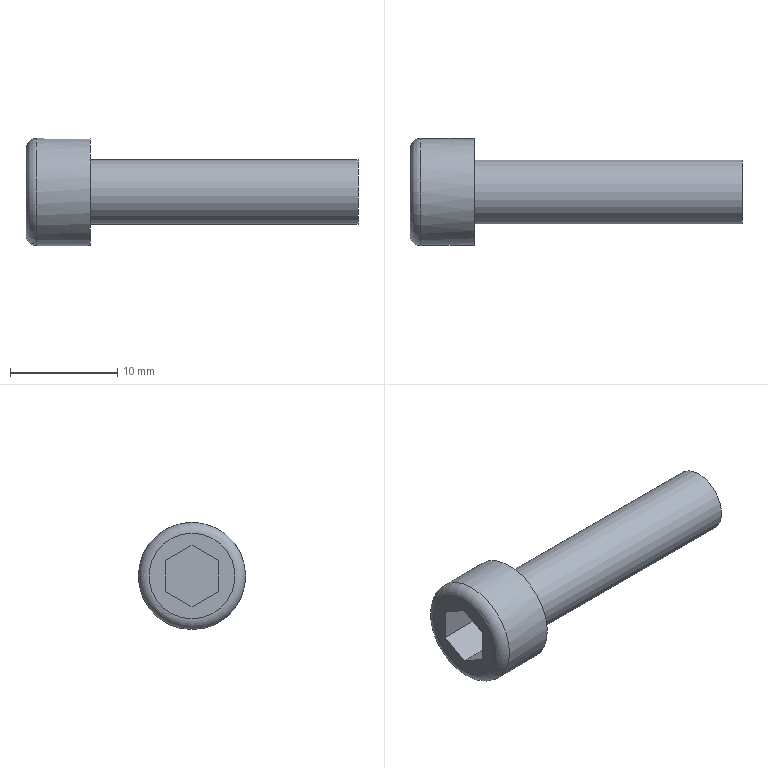Part | STEP file | Tube necking machine_id230_x_t | 1 solid | 13 faces | box 31 x 10 x 10 mm | volume 1086 mm3 | plane 10 | cylinder 2 | torus 1 | commonest cylinder face diameters 6 x1 10 x1
STEP:
#1=CARTESIAN_POINT('',(0.,0.,0.));
#2=DIRECTION('',(0.,0.,1.));
#3=DIRECTION('',(1.,0.,0.));
#4=AXIS2_PLACEMENT_3D('',#1,#2,#3);
#5=CARTESIAN_POINT('',(-139.5,-84.,264.));
#6=VERTEX_POINT('',#5);
#7=CARTESIAN_POINT('',(-139.5,-84.,260.));
#8=DIRECTION('',(-1.,0.,0.));
#9=DIRECTION('',(0.,0.,1.));
#10=AXIS2_PLACEMENT_3D('',#7,#8,#9);
#11=CIRCLE('',#10,4.);
#12=CARTESIAN_POINT('',(-139.5,-84.,255.));
#13=DIRECTION('',(1.,0.,0.));
#14=DIRECTION('',(0.,0.,1.));
#15=AXIS2_PLACEMENT_3D('',#12,#13,#14);
#16=PLANE('',#15);
#17=CARTESIAN_POINT('',(9.,0.));
#18=CARTESIAN_POINT('',(9.,-6.928));
#19=CARTESIAN_POINT('',(3.,-3.464));
#20=CARTESIAN_POINT('',(-3.,0.));
#21=CARTESIAN_POINT('',(3.,3.464));
#22=CARTESIAN_POINT('',(9.,6.928));
#23=CARTESIAN_POINT('',(9.,0.));
#24=(BOUNDED_CURVE()B_SPLINE_CURVE(2,(#17,#18,#19,#20,#21,#22,#23),.UNSPECIFIED.,.T.,.F.)B_SPLINE_CURVE_WITH_KNOTS((1,2,2,2,2,1),(-2.094,0.,2.094,4.189,6.283,8.378),.UNSPECIFIED.)CURVE()GEOMETRIC_REPRESENTATION_ITEM()RATIONAL_B_SPLINE_CURVE((1.,0.5,1.,0.5,1.,0.5,1.))REPRESENTATION_ITEM(''));
#25=(GEOMETRIC_REPRESENTATION_CONTEXT(2)PARAMETRIC_REPRESENTATION_CONTEXT()REPRESENTATION_CONTEXT('',''));
#26=DEFINITIONAL_REPRESENTATION('',(#24),#25);
#27=PCURVE('',#16,#26);
#28=CARTESIAN_POINT('',(-138.5,-84.,260.));
#29=DIRECTION('',(1.,0.,0.));
#30=DIRECTION('',(0.,0.,1.));
#31=AXIS2_PLACEMENT_3D('',#28,#29,#30);
#32=TOROIDAL_SURFACE('',#31,4.,1.);
#33=CARTESIAN_POINT('',(6.283,4.712));
#34=DIRECTION('',(-1.,0.));
#35=VECTOR('',#34,1.);
#36=LINE('',#33,#35);
#37=(GEOMETRIC_REPRESENTATION_CONTEXT(2)PARAMETRIC_REPRESENTATION_CONTEXT()REPRESENTATION_CONTEXT('',''));
#38=DEFINITIONAL_REPRESENTATION('',(#36),#37);
#39=PCURVE('',#32,#38);
#40=SURFACE_CURVE('',#11,(#27,#39),.PCURVE_S1.);
#41=EDGE_CURVE('',#6,#6,#40,.T.);
#42=ORIENTED_EDGE('',*,*,#41,.T.);
#43=EDGE_LOOP('',(#42));
#44=FACE_BOUND('',#43,.T.);
#45=CARTESIAN_POINT('',(-139.5,-81.5,258.557));
#46=VERTEX_POINT('',#45);
#47=CARTESIAN_POINT('',(-139.5,-81.5,261.443));
#48=VERTEX_POINT('',#47);
#49=CARTESIAN_POINT('',(-139.5,-81.5,261.443));
#50=DIRECTION('',(0.,0.,1.));
#51=VECTOR('',#50,1.);
#52=LINE('',#49,#51);
#53=CARTESIAN_POINT('',(6.443,-2.5));
#54=DIRECTION('',(1.,0.));
#55=VECTOR('',#54,1.);
#56=LINE('',#53,#55);
#57=(GEOMETRIC_REPRESENTATION_CONTEXT(2)PARAMETRIC_REPRESENTATION_CONTEXT()REPRESENTATION_CONTEXT('',''));
#58=DEFINITIONAL_REPRESENTATION('',(#56),#57);
#59=PCURVE('',#16,#58);
#60=CARTESIAN_POINT('',(-135.54,-81.5,261.443));
#61=DIRECTION('',(0.,-1.,0.));
#62=DIRECTION('',(1.,0.,0.));
#63=AXIS2_PLACEMENT_3D('',#60,#61,#62);
#64=PLANE('',#63);
#65=CARTESIAN_POINT('',(-3.96,0.));
#66=DIRECTION('',(0.,1.));
#67=VECTOR('',#66,1.);
#68=LINE('',#65,#67);
#69=(GEOMETRIC_REPRESENTATION_CONTEXT(2)PARAMETRIC_REPRESENTATION_CONTEXT()REPRESENTATION_CONTEXT('',''));
#70=DEFINITIONAL_REPRESENTATION('',(#68),#69);
#71=PCURVE('',#64,#70);
#72=SURFACE_CURVE('',#52,(#59,#71),.PCURVE_S1.);
#73=EDGE_CURVE('',#46,#48,#72,.T.);
#74=ORIENTED_EDGE('',*,*,#73,.T.);
#75=CARTESIAN_POINT('',(-139.5,-84.,262.887));
#76=VERTEX_POINT('',#75);
#77=CARTESIAN_POINT('',(-139.5,-84.,262.887));
#78=DIRECTION('',(0.,-0.866,0.5));
#79=VECTOR('',#78,1.);
#80=LINE('',#77,#79);
#81=CARTESIAN_POINT('',(7.887,0.));
#82=DIRECTION('',(0.5,0.866));
#83=VECTOR('',#82,1.);
#84=LINE('',#81,#83);
#85=(GEOMETRIC_REPRESENTATION_CONTEXT(2)PARAMETRIC_REPRESENTATION_CONTEXT()REPRESENTATION_CONTEXT('',''));
#86=DEFINITIONAL_REPRESENTATION('',(#84),#85);
#87=PCURVE('',#16,#86);
#88=CARTESIAN_POINT('',(-135.54,-84.,262.887));
#89=DIRECTION('',(0.,-0.5,-0.866));
#90=DIRECTION('',(0.,0.866,-0.5));
#91=AXIS2_PLACEMENT_3D('',#88,#89,#90);
#92=PLANE('',#91);
#93=CARTESIAN_POINT('',(0.,-3.96));
#94=DIRECTION('',(-1.,0.));
#95=VECTOR('',#94,1.);
#96=LINE('',#93,#95);
#97=(GEOMETRIC_REPRESENTATION_CONTEXT(2)PARAMETRIC_REPRESENTATION_CONTEXT()REPRESENTATION_CONTEXT('',''));
#98=DEFINITIONAL_REPRESENTATION('',(#96),#97);
#99=PCURVE('',#92,#98);
#100=SURFACE_CURVE('',#80,(#87,#99),.PCURVE_S1.);
#101=EDGE_CURVE('',#48,#76,#100,.T.);
#102=ORIENTED_EDGE('',*,*,#101,.T.);
#103=CARTESIAN_POINT('',(-139.5,-86.5,261.443));
#104=VERTEX_POINT('',#103);
#105=CARTESIAN_POINT('',(-139.5,-86.5,261.443));
#106=DIRECTION('',(0.,-0.866,-0.5));
#107=VECTOR('',#106,1.);
#108=LINE('',#105,#107);
#109=CARTESIAN_POINT('',(6.443,2.5));
#110=DIRECTION('',(-0.5,0.866));
#111=VECTOR('',#110,1.);
#112=LINE('',#109,#111);
#113=(GEOMETRIC_REPRESENTATION_CONTEXT(2)PARAMETRIC_REPRESENTATION_CONTEXT()REPRESENTATION_CONTEXT('',''));
#114=DEFINITIONAL_REPRESENTATION('',(#112),#113);
#115=PCURVE('',#16,#114);
#116=CARTESIAN_POINT('',(-135.54,-86.5,261.443));
#117=DIRECTION('',(0.,0.5,-0.866));
#118=DIRECTION('',(0.,0.866,0.5));
#119=AXIS2_PLACEMENT_3D('',#116,#117,#118);
#120=PLANE('',#119);
#121=CARTESIAN_POINT('',(0.,-3.96));
#122=DIRECTION('',(-1.,0.));
#123=VECTOR('',#122,1.);
#124=LINE('',#121,#123);
#125=(GEOMETRIC_REPRESENTATION_CONTEXT(2)PARAMETRIC_REPRESENTATION_CONTEXT()REPRESENTATION_CONTEXT('',''));
#126=DEFINITIONAL_REPRESENTATION('',(#124),#125);
#127=PCURVE('',#120,#126);
#128=SURFACE_CURVE('',#108,(#115,#127),.PCURVE_S1.);
#129=EDGE_CURVE('',#76,#104,#128,.T.);
#130=ORIENTED_EDGE('',*,*,#129,.T.);
#131=CARTESIAN_POINT('',(-139.5,-86.5,258.557));
#132=VERTEX_POINT('',#131);
#133=CARTESIAN_POINT('',(-139.5,-86.5,258.557));
#134=DIRECTION('',(0.,0.,-1.));
#135=VECTOR('',#134,1.);
#136=LINE('',#133,#135);
#137=CARTESIAN_POINT('',(3.557,2.5));
#138=DIRECTION('',(-1.,0.));
#139=VECTOR('',#138,1.);
#140=LINE('',#137,#139);
#141=(GEOMETRIC_REPRESENTATION_CONTEXT(2)PARAMETRIC_REPRESENTATION_CONTEXT()REPRESENTATION_CONTEXT('',''));
#142=DEFINITIONAL_REPRESENTATION('',(#140),#141);
#143=PCURVE('',#16,#142);
#144=CARTESIAN_POINT('',(-135.54,-86.5,258.557));
#145=DIRECTION('',(0.,1.,0.));
#146=DIRECTION('',(0.,0.,1.));
#147=AXIS2_PLACEMENT_3D('',#144,#145,#146);
#148=PLANE('',#147);
#149=CARTESIAN_POINT('',(0.,-3.96));
#150=DIRECTION('',(-1.,0.));
#151=VECTOR('',#150,1.);
#152=LINE('',#149,#151);
#153=(GEOMETRIC_REPRESENTATION_CONTEXT(2)PARAMETRIC_REPRESENTATION_CONTEXT()REPRESENTATION_CONTEXT('',''));
#154=DEFINITIONAL_REPRESENTATION('',(#152),#153);
#155=PCURVE('',#148,#154);
#156=SURFACE_CURVE('',#136,(#143,#155),.PCURVE_S1.);
#157=EDGE_CURVE('',#104,#132,#156,.T.);
#158=ORIENTED_EDGE('',*,*,#157,.T.);
#159=CARTESIAN_POINT('',(-139.5,-84.,257.113));
#160=VERTEX_POINT('',#159);
#161=CARTESIAN_POINT('',(-139.5,-84.,257.113));
#162=DIRECTION('',(0.,0.866,-0.5));
#163=VECTOR('',#162,1.);
#164=LINE('',#161,#163);
#165=CARTESIAN_POINT('',(2.113,0.));
#166=DIRECTION('',(-0.5,-0.866));
#167=VECTOR('',#166,1.);
#168=LINE('',#165,#167);
#169=(GEOMETRIC_REPRESENTATION_CONTEXT(2)PARAMETRIC_REPRESENTATION_CONTEXT()REPRESENTATION_CONTEXT('',''));
#170=DEFINITIONAL_REPRESENTATION('',(#168),#169);
#171=PCURVE('',#16,#170);
#172=CARTESIAN_POINT('',(-135.54,-84.,257.113));
#173=DIRECTION('',(0.,0.5,0.866));
#174=DIRECTION('',(0.,-0.866,0.5));
#175=AXIS2_PLACEMENT_3D('',#172,#173,#174);
#176=PLANE('',#175);
#177=CARTESIAN_POINT('',(0.,-3.96));
#178=DIRECTION('',(-1.,0.));
#179=VECTOR('',#178,1.);
#180=LINE('',#177,#179);
#181=(GEOMETRIC_REPRESENTATION_CONTEXT(2)PARAMETRIC_REPRESENTATION_CONTEXT()REPRESENTATION_CONTEXT('',''));
#182=DEFINITIONAL_REPRESENTATION('',(#180),#181);
#183=PCURVE('',#176,#182);
#184=SURFACE_CURVE('',#164,(#171,#183),.PCURVE_S1.);
#185=EDGE_CURVE('',#132,#160,#184,.T.);
#186=ORIENTED_EDGE('',*,*,#185,.T.);
#187=CARTESIAN_POINT('',(-139.5,-81.5,258.557));
#188=DIRECTION('',(0.,0.866,0.5));
#189=VECTOR('',#188,1.);
#190=LINE('',#187,#189);
#191=CARTESIAN_POINT('',(3.557,-2.5));
#192=DIRECTION('',(0.5,-0.866));
#193=VECTOR('',#192,1.);
#194=LINE('',#191,#193);
#195=(GEOMETRIC_REPRESENTATION_CONTEXT(2)PARAMETRIC_REPRESENTATION_CONTEXT()REPRESENTATION_CONTEXT('',''));
#196=DEFINITIONAL_REPRESENTATION('',(#194),#195);
#197=PCURVE('',#16,#196);
#198=CARTESIAN_POINT('',(-135.54,-81.5,258.557));
#199=DIRECTION('',(0.,-0.5,0.866));
#200=DIRECTION('',(0.,-0.866,-0.5));
#201=AXIS2_PLACEMENT_3D('',#198,#199,#200);
#202=PLANE('',#201);
#203=CARTESIAN_POINT('',(0.,-3.96));
#204=DIRECTION('',(-1.,0.));
#205=VECTOR('',#204,1.);
#206=LINE('',#203,#205);
#207=(GEOMETRIC_REPRESENTATION_CONTEXT(2)PARAMETRIC_REPRESENTATION_CONTEXT()REPRESENTATION_CONTEXT('',''));
#208=DEFINITIONAL_REPRESENTATION('',(#206),#207);
#209=PCURVE('',#202,#208);
#210=SURFACE_CURVE('',#190,(#197,#209),.PCURVE_S1.);
#211=EDGE_CURVE('',#160,#46,#210,.T.);
#212=ORIENTED_EDGE('',*,*,#211,.T.);
#213=EDGE_LOOP('',(#74,#102,#130,#158,#186,#212));
#214=FACE_BOUND('',#213,.T.);
#215=ADVANCED_FACE('',(#44,#214),#16,.F.);
#216=CARTESIAN_POINT('',(-138.5,-84.,265.));
#217=VERTEX_POINT('',#216);
#218=CARTESIAN_POINT('',(-138.5,-84.,255.));
#219=VERTEX_POINT('',#218);
#220=CARTESIAN_POINT('',(-138.5,-84.,260.));
#221=DIRECTION('',(1.,0.,0.));
#222=DIRECTION('',(0.,0.,1.));
#223=AXIS2_PLACEMENT_3D('',#220,#221,#222);
#224=CIRCLE('',#223,5.);
#225=CARTESIAN_POINT('',(-134.6,-84.,260.));
#226=DIRECTION('',(-1.,0.,0.));
#227=DIRECTION('',(0.,0.,-1.));
#228=AXIS2_PLACEMENT_3D('',#225,#226,#227);
#229=CYLINDRICAL_SURFACE('',#228,5.);
#230=CARTESIAN_POINT('',(3.142,3.9));
#231=DIRECTION('',(-1.,0.));
#232=VECTOR('',#231,1.);
#233=LINE('',#230,#232);
#234=(GEOMETRIC_REPRESENTATION_CONTEXT(2)PARAMETRIC_REPRESENTATION_CONTEXT()REPRESENTATION_CONTEXT('',''));
#235=DEFINITIONAL_REPRESENTATION('',(#233),#234);
#236=PCURVE('',#229,#235);
#237=CARTESIAN_POINT('',(0.,6.283));
#238=DIRECTION('',(1.,0.));
#239=VECTOR('',#238,1.);
#240=LINE('',#237,#239);
#241=(GEOMETRIC_REPRESENTATION_CONTEXT(2)PARAMETRIC_REPRESENTATION_CONTEXT()REPRESENTATION_CONTEXT('',''));
#242=DEFINITIONAL_REPRESENTATION('',(#240),#241);
#243=PCURVE('',#32,#242);
#244=SURFACE_CURVE('',#224,(#236,#243),.PCURVE_S1.);
#245=EDGE_CURVE('',#217,#219,#244,.T.);
#246=ORIENTED_EDGE('',*,*,#245,.T.);
#247=CARTESIAN_POINT('',(-133.5,-84.,255.));
#248=VERTEX_POINT('',#247);
#249=CARTESIAN_POINT('',(-133.5,-84.,255.));
#250=CARTESIAN_POINT('',(-138.5,-84.,255.));
#251=B_SPLINE_CURVE_WITH_KNOTS('',1,(#249,#250),.UNSPECIFIED.,.F.,.F.,(2,2),(-1.1,3.9),.PIECEWISE_BEZIER_KNOTS.);
#252=CARTESIAN_POINT('',(0.,0.));
#253=DIRECTION('',(0.,1.));
#254=VECTOR('',#253,1.);
#255=LINE('',#252,#254);
#256=(GEOMETRIC_REPRESENTATION_CONTEXT(2)PARAMETRIC_REPRESENTATION_CONTEXT()REPRESENTATION_CONTEXT('',''));
#257=DEFINITIONAL_REPRESENTATION('',(#255),#256);
#258=PCURVE('',#229,#257);
#259=CARTESIAN_POINT('',(6.283,0.));
#260=DIRECTION('',(0.,1.));
#261=VECTOR('',#260,1.);
#262=LINE('',#259,#261);
#263=(GEOMETRIC_REPRESENTATION_CONTEXT(2)PARAMETRIC_REPRESENTATION_CONTEXT()REPRESENTATION_CONTEXT('',''));
#264=DEFINITIONAL_REPRESENTATION('',(#262),#263);
#265=PCURVE('',#229,#264);
#266=SEAM_CURVE('',#251,(#258,#265),.PCURVE_S1.);
#267=EDGE_CURVE('',#248,#219,#266,.T.);
#268=ORIENTED_EDGE('',*,*,#267,.F.);
#269=CARTESIAN_POINT('',(-133.5,-84.,260.));
#270=DIRECTION('',(-1.,0.,0.));
#271=DIRECTION('',(0.,0.,-1.));
#272=AXIS2_PLACEMENT_3D('',#269,#270,#271);
#273=CIRCLE('',#272,5.);
#274=CARTESIAN_POINT('',(0.,-1.1));
#275=DIRECTION('',(1.,0.));
#276=VECTOR('',#275,1.);
#277=LINE('',#274,#276);
#278=(GEOMETRIC_REPRESENTATION_CONTEXT(2)PARAMETRIC_REPRESENTATION_CONTEXT()REPRESENTATION_CONTEXT('',''));
#279=DEFINITIONAL_REPRESENTATION('',(#277),#278);
#280=PCURVE('',#229,#279);
#281=CARTESIAN_POINT('',(-133.5,-84.,257.));
#282=DIRECTION('',(-1.,0.,0.));
#283=DIRECTION('',(0.,0.,-1.));
#284=AXIS2_PLACEMENT_3D('',#281,#282,#283);
#285=PLANE('',#284);
#286=CARTESIAN_POINT('',(-3.,0.));
#287=DIRECTION('',(1.,0.));
#288=AXIS2_PLACEMENT_2D('',#286,#287);
#289=CIRCLE('',#288,5.);
#290=(GEOMETRIC_REPRESENTATION_CONTEXT(2)PARAMETRIC_REPRESENTATION_CONTEXT()REPRESENTATION_CONTEXT('',''));
#291=DEFINITIONAL_REPRESENTATION('',(#289),#290);
#292=PCURVE('',#285,#291);
#293=SURFACE_CURVE('',#273,(#280,#292),.PCURVE_S1.);
#294=EDGE_CURVE('',#248,#248,#293,.T.);
#295=ORIENTED_EDGE('',*,*,#294,.T.);
#296=ORIENTED_EDGE('',*,*,#267,.T.);
#297=CARTESIAN_POINT('',(-138.5,-84.,260.));
#298=DIRECTION('',(1.,0.,0.));
#299=DIRECTION('',(0.,0.,1.));
#300=AXIS2_PLACEMENT_3D('',#297,#298,#299);
#301=CIRCLE('',#300,5.);
#302=CARTESIAN_POINT('',(9.425,3.9));
#303=DIRECTION('',(-1.,0.));
#304=VECTOR('',#303,1.);
#305=LINE('',#302,#304);
#306=(GEOMETRIC_REPRESENTATION_CONTEXT(2)PARAMETRIC_REPRESENTATION_CONTEXT()REPRESENTATION_CONTEXT('',''));
#307=DEFINITIONAL_REPRESENTATION('',(#305),#306);
#308=PCURVE('',#229,#307);
#309=CARTESIAN_POINT('',(0.,6.283));
#310=DIRECTION('',(1.,0.));
#311=VECTOR('',#310,1.);
#312=LINE('',#309,#311);
#313=(GEOMETRIC_REPRESENTATION_CONTEXT(2)PARAMETRIC_REPRESENTATION_CONTEXT()REPRESENTATION_CONTEXT('',''));
#314=DEFINITIONAL_REPRESENTATION('',(#312),#313);
#315=PCURVE('',#32,#314);
#316=SURFACE_CURVE('',#301,(#308,#315),.PCURVE_S1.);
#317=EDGE_CURVE('',#219,#217,#316,.T.);
#318=ORIENTED_EDGE('',*,*,#317,.T.);
#319=EDGE_LOOP('',(#246,#268,#295,#296,#318));
#320=FACE_BOUND('',#319,.T.);
#321=ADVANCED_FACE('',(#320),#229,.T.);
#322=ORIENTED_EDGE('',*,*,#294,.F.);
#323=EDGE_LOOP('',(#322));
#324=FACE_BOUND('',#323,.T.);
#325=CARTESIAN_POINT('',(-133.5,-84.,257.));
#326=VERTEX_POINT('',#325);
#327=CARTESIAN_POINT('',(-133.5,-84.,260.));
#328=DIRECTION('',(-1.,0.,0.));
#329=DIRECTION('',(0.,0.,-1.));
#330=AXIS2_PLACEMENT_3D('',#327,#328,#329);
#331=CIRCLE('',#330,3.);
#332=CARTESIAN_POINT('',(-3.,0.));
#333=DIRECTION('',(1.,0.));
#334=AXIS2_PLACEMENT_2D('',#332,#333);
#335=CIRCLE('',#334,3.);
#336=(GEOMETRIC_REPRESENTATION_CONTEXT(2)PARAMETRIC_REPRESENTATION_CONTEXT()REPRESENTATION_CONTEXT('',''));
#337=DEFINITIONAL_REPRESENTATION('',(#335),#336);
#338=PCURVE('',#285,#337);
#339=CARTESIAN_POINT('',(-134.6,-84.,260.));
#340=DIRECTION('',(-1.,0.,0.));
#341=DIRECTION('',(0.,0.,-1.));
#342=AXIS2_PLACEMENT_3D('',#339,#340,#341);
#343=CYLINDRICAL_SURFACE('',#342,3.);
#344=CARTESIAN_POINT('',(0.,-1.1));
#345=DIRECTION('',(1.,0.));
#346=VECTOR('',#345,1.);
#347=LINE('',#344,#346);
#348=(GEOMETRIC_REPRESENTATION_CONTEXT(2)PARAMETRIC_REPRESENTATION_CONTEXT()REPRESENTATION_CONTEXT('',''));
#349=DEFINITIONAL_REPRESENTATION('',(#347),#348);
#350=PCURVE('',#343,#349);
#351=SURFACE_CURVE('',#331,(#338,#350),.PCURVE_S1.);
#352=EDGE_CURVE('',#326,#326,#351,.T.);
#353=ORIENTED_EDGE('',*,*,#352,.T.);
#354=EDGE_LOOP('',(#353));
#355=FACE_BOUND('',#354,.T.);
#356=ADVANCED_FACE('',(#324,#355),#285,.F.);
#357=ORIENTED_EDGE('',*,*,#352,.F.);
#358=CARTESIAN_POINT('',(-108.5,-84.,257.));
#359=VERTEX_POINT('',#358);
#360=CARTESIAN_POINT('',(-108.5,-84.,257.));
#361=CARTESIAN_POINT('',(-133.5,-84.,257.));
#362=B_SPLINE_CURVE_WITH_KNOTS('',1,(#360,#361),.UNSPECIFIED.,.F.,.F.,(2,2),(-26.1,-1.1),.PIECEWISE_BEZIER_KNOTS.);
#363=CARTESIAN_POINT('',(0.,0.));
#364=DIRECTION('',(0.,1.));
#365=VECTOR('',#364,1.);
#366=LINE('',#363,#365);
#367=(GEOMETRIC_REPRESENTATION_CONTEXT(2)PARAMETRIC_REPRESENTATION_CONTEXT()REPRESENTATION_CONTEXT('',''));
#368=DEFINITIONAL_REPRESENTATION('',(#366),#367);
#369=PCURVE('',#343,#368);
#370=CARTESIAN_POINT('',(6.283,0.));
#371=DIRECTION('',(0.,1.));
#372=VECTOR('',#371,1.);
#373=LINE('',#370,#372);
#374=(GEOMETRIC_REPRESENTATION_CONTEXT(2)PARAMETRIC_REPRESENTATION_CONTEXT()REPRESENTATION_CONTEXT('',''));
#375=DEFINITIONAL_REPRESENTATION('',(#373),#374);
#376=PCURVE('',#343,#375);
#377=SEAM_CURVE('',#362,(#369,#376),.PCURVE_S1.);
#378=EDGE_CURVE('',#359,#326,#377,.T.);
#379=ORIENTED_EDGE('',*,*,#378,.F.);
#380=CARTESIAN_POINT('',(-108.5,-84.,260.));
#381=DIRECTION('',(-1.,0.,0.));
#382=DIRECTION('',(0.,0.,-1.));
#383=AXIS2_PLACEMENT_3D('',#380,#381,#382);
#384=CIRCLE('',#383,3.);
#385=CARTESIAN_POINT('',(0.,-26.1));
#386=DIRECTION('',(1.,0.));
#387=VECTOR('',#386,1.);
#388=LINE('',#385,#387);
#389=(GEOMETRIC_REPRESENTATION_CONTEXT(2)PARAMETRIC_REPRESENTATION_CONTEXT()REPRESENTATION_CONTEXT('',''));
#390=DEFINITIONAL_REPRESENTATION('',(#388),#389);
#391=PCURVE('',#343,#390);
#392=CARTESIAN_POINT('',(-108.5,-84.,260.));
#393=DIRECTION('',(-1.,0.,0.));
#394=DIRECTION('',(0.,0.,-1.));
#395=AXIS2_PLACEMENT_3D('',#392,#393,#394);
#396=PLANE('',#395);
#397=CARTESIAN_POINT('',(0.,0.));
#398=DIRECTION('',(1.,0.));
#399=AXIS2_PLACEMENT_2D('',#397,#398);
#400=CIRCLE('',#399,3.);
#401=(GEOMETRIC_REPRESENTATION_CONTEXT(2)PARAMETRIC_REPRESENTATION_CONTEXT()REPRESENTATION_CONTEXT('',''));
#402=DEFINITIONAL_REPRESENTATION('',(#400),#401);
#403=PCURVE('',#396,#402);
#404=SURFACE_CURVE('',#384,(#391,#403),.PCURVE_S1.);
#405=EDGE_CURVE('',#359,#359,#404,.T.);
#406=ORIENTED_EDGE('',*,*,#405,.T.);
#407=ORIENTED_EDGE('',*,*,#378,.T.);
#408=EDGE_LOOP('',(#357,#379,#406,#407));
#409=FACE_BOUND('',#408,.T.);
#410=ADVANCED_FACE('',(#409),#343,.T.);
#411=ORIENTED_EDGE('',*,*,#405,.F.);
#412=EDGE_LOOP('',(#411));
#413=FACE_BOUND('',#412,.T.);
#414=ADVANCED_FACE('',(#413),#396,.F.);
#415=ORIENTED_EDGE('',*,*,#73,.F.);
#416=CARTESIAN_POINT('',(-135.54,-81.5,258.557));
#417=VERTEX_POINT('',#416);
#418=CARTESIAN_POINT('',(-135.54,-81.5,258.557));
#419=DIRECTION('',(-1.,0.,0.));
#420=VECTOR('',#419,1.);
#421=LINE('',#418,#420);
#422=CARTESIAN_POINT('',(0.,-2.887));
#423=DIRECTION('',(-1.,0.));
#424=VECTOR('',#423,1.);
#425=LINE('',#422,#424);
#426=(GEOMETRIC_REPRESENTATION_CONTEXT(2)PARAMETRIC_REPRESENTATION_CONTEXT()REPRESENTATION_CONTEXT('',''));
#427=DEFINITIONAL_REPRESENTATION('',(#425),#426);
#428=PCURVE('',#64,#427);
#429=CARTESIAN_POINT('',(0.,0.));
#430=DIRECTION('',(0.,-1.));
#431=VECTOR('',#430,1.);
#432=LINE('',#429,#431);
#433=(GEOMETRIC_REPRESENTATION_CONTEXT(2)PARAMETRIC_REPRESENTATION_CONTEXT()REPRESENTATION_CONTEXT('',''));
#434=DEFINITIONAL_REPRESENTATION('',(#432),#433);
#435=PCURVE('',#202,#434);
#436=SURFACE_CURVE('',#421,(#428,#435),.PCURVE_S1.);
#437=EDGE_CURVE('',#417,#46,#436,.T.);
#438=ORIENTED_EDGE('',*,*,#437,.F.);
#439=CARTESIAN_POINT('',(-135.54,-81.5,261.443));
#440=VERTEX_POINT('',#439);
#441=CARTESIAN_POINT('',(-135.54,-81.5,261.443));
#442=DIRECTION('',(0.,0.,-1.));
#443=VECTOR('',#442,1.);
#444=LINE('',#441,#443);
#445=CARTESIAN_POINT('',(0.,0.));
#446=DIRECTION('',(0.,-1.));
#447=VECTOR('',#446,1.);
#448=LINE('',#445,#447);
#449=(GEOMETRIC_REPRESENTATION_CONTEXT(2)PARAMETRIC_REPRESENTATION_CONTEXT()REPRESENTATION_CONTEXT('',''));
#450=DEFINITIONAL_REPRESENTATION('',(#448),#449);
#451=PCURVE('',#64,#450);
#452=CARTESIAN_POINT('',(-135.54,-84.,260.));
#453=DIRECTION('',(1.,0.,0.));
#454=DIRECTION('',(0.,0.,1.));
#455=AXIS2_PLACEMENT_3D('',#452,#453,#454);
#456=PLANE('',#455);
#457=CARTESIAN_POINT('',(1.443,-2.5));
#458=DIRECTION('',(-1.,0.));
#459=VECTOR('',#458,1.);
#460=LINE('',#457,#459);
#461=(GEOMETRIC_REPRESENTATION_CONTEXT(2)PARAMETRIC_REPRESENTATION_CONTEXT()REPRESENTATION_CONTEXT('',''));
#462=DEFINITIONAL_REPRESENTATION('',(#460),#461);
#463=PCURVE('',#456,#462);
#464=SURFACE_CURVE('',#444,(#451,#463),.PCURVE_S1.);
#465=EDGE_CURVE('',#440,#417,#464,.T.);
#466=ORIENTED_EDGE('',*,*,#465,.F.);
#467=CARTESIAN_POINT('',(-135.54,-81.5,261.443));
#468=DIRECTION('',(-1.,0.,0.));
#469=VECTOR('',#468,1.);
#470=LINE('',#467,#469);
#471=CARTESIAN_POINT('',(0.,0.));
#472=DIRECTION('',(-1.,0.));
#473=VECTOR('',#472,1.);
#474=LINE('',#471,#473);
#475=(GEOMETRIC_REPRESENTATION_CONTEXT(2)PARAMETRIC_REPRESENTATION_CONTEXT()REPRESENTATION_CONTEXT('',''));
#476=DEFINITIONAL_REPRESENTATION('',(#474),#475);
#477=PCURVE('',#64,#476);
#478=CARTESIAN_POINT('',(2.887,0.));
#479=DIRECTION('',(0.,-1.));
#480=VECTOR('',#479,1.);
#481=LINE('',#478,#480);
#482=(GEOMETRIC_REPRESENTATION_CONTEXT(2)PARAMETRIC_REPRESENTATION_CONTEXT()REPRESENTATION_CONTEXT('',''));
#483=DEFINITIONAL_REPRESENTATION('',(#481),#482);
#484=PCURVE('',#92,#483);
#485=SURFACE_CURVE('',#470,(#477,#484),.PCURVE_S1.);
#486=EDGE_CURVE('',#440,#48,#485,.T.);
#487=ORIENTED_EDGE('',*,*,#486,.T.);
#488=EDGE_LOOP('',(#415,#438,#466,#487));
#489=FACE_BOUND('',#488,.T.);
#490=ADVANCED_FACE('',(#489),#64,.T.);
#491=ORIENTED_EDGE('',*,*,#211,.F.);
#492=CARTESIAN_POINT('',(-135.54,-84.,257.113));
#493=VERTEX_POINT('',#492);
#494=CARTESIAN_POINT('',(-135.54,-84.,257.113));
#495=DIRECTION('',(-1.,0.,0.));
#496=VECTOR('',#495,1.);
#497=LINE('',#494,#496);
#498=CARTESIAN_POINT('',(2.887,0.));
#499=DIRECTION('',(0.,-1.));
#500=VECTOR('',#499,1.);
#501=LINE('',#498,#500);
#502=(GEOMETRIC_REPRESENTATION_CONTEXT(2)PARAMETRIC_REPRESENTATION_CONTEXT()REPRESENTATION_CONTEXT('',''));
#503=DEFINITIONAL_REPRESENTATION('',(#501),#502);
#504=PCURVE('',#202,#503);
#505=CARTESIAN_POINT('',(0.,0.));
#506=DIRECTION('',(0.,-1.));
#507=VECTOR('',#506,1.);
#508=LINE('',#505,#507);
#509=(GEOMETRIC_REPRESENTATION_CONTEXT(2)PARAMETRIC_REPRESENTATION_CONTEXT()REPRESENTATION_CONTEXT('',''));
#510=DEFINITIONAL_REPRESENTATION('',(#508),#509);
#511=PCURVE('',#176,#510);
#512=SURFACE_CURVE('',#497,(#504,#511),.PCURVE_S1.);
#513=EDGE_CURVE('',#493,#160,#512,.T.);
#514=ORIENTED_EDGE('',*,*,#513,.F.);
#515=CARTESIAN_POINT('',(-135.54,-81.5,258.557));
#516=DIRECTION('',(0.,-0.866,-0.5));
#517=VECTOR('',#516,1.);
#518=LINE('',#515,#517);
#519=CARTESIAN_POINT('',(0.,0.));
#520=DIRECTION('',(1.,0.));
#521=VECTOR('',#520,1.);
#522=LINE('',#519,#521);
#523=(GEOMETRIC_REPRESENTATION_CONTEXT(2)PARAMETRIC_REPRESENTATION_CONTEXT()REPRESENTATION_CONTEXT('',''));
#524=DEFINITIONAL_REPRESENTATION('',(#522),#523);
#525=PCURVE('',#202,#524);
#526=CARTESIAN_POINT('',(-1.443,-2.5));
#527=DIRECTION('',(-0.5,0.866));
#528=VECTOR('',#527,1.);
#529=LINE('',#526,#528);
#530=(GEOMETRIC_REPRESENTATION_CONTEXT(2)PARAMETRIC_REPRESENTATION_CONTEXT()REPRESENTATION_CONTEXT('',''));
#531=DEFINITIONAL_REPRESENTATION('',(#529),#530);
#532=PCURVE('',#456,#531);
#533=SURFACE_CURVE('',#518,(#525,#532),.PCURVE_S1.);
#534=EDGE_CURVE('',#417,#493,#533,.T.);
#535=ORIENTED_EDGE('',*,*,#534,.F.);
#536=ORIENTED_EDGE('',*,*,#437,.T.);
#537=EDGE_LOOP('',(#491,#514,#535,#536));
#538=FACE_BOUND('',#537,.T.);
#539=ADVANCED_FACE('',(#538),#202,.T.);
#540=ORIENTED_EDGE('',*,*,#185,.F.);
#541=CARTESIAN_POINT('',(-135.54,-86.5,258.557));
#542=VERTEX_POINT('',#541);
#543=CARTESIAN_POINT('',(-135.54,-86.5,258.557));
#544=DIRECTION('',(-1.,0.,0.));
#545=VECTOR('',#544,1.);
#546=LINE('',#543,#545);
#547=CARTESIAN_POINT('',(2.887,0.));
#548=DIRECTION('',(0.,-1.));
#549=VECTOR('',#548,1.);
#550=LINE('',#547,#549);
#551=(GEOMETRIC_REPRESENTATION_CONTEXT(2)PARAMETRIC_REPRESENTATION_CONTEXT()REPRESENTATION_CONTEXT('',''));
#552=DEFINITIONAL_REPRESENTATION('',(#550),#551);
#553=PCURVE('',#176,#552);
#554=CARTESIAN_POINT('',(0.,0.));
#555=DIRECTION('',(0.,-1.));
#556=VECTOR('',#555,1.);
#557=LINE('',#554,#556);
#558=(GEOMETRIC_REPRESENTATION_CONTEXT(2)PARAMETRIC_REPRESENTATION_CONTEXT()REPRESENTATION_CONTEXT('',''));
#559=DEFINITIONAL_REPRESENTATION('',(#557),#558);
#560=PCURVE('',#148,#559);
#561=SURFACE_CURVE('',#546,(#553,#560),.PCURVE_S1.);
#562=EDGE_CURVE('',#542,#132,#561,.T.);
#563=ORIENTED_EDGE('',*,*,#562,.F.);
#564=CARTESIAN_POINT('',(-135.54,-84.,257.113));
#565=DIRECTION('',(0.,-0.866,0.5));
#566=VECTOR('',#565,1.);
#567=LINE('',#564,#566);
#568=CARTESIAN_POINT('',(0.,0.));
#569=DIRECTION('',(1.,0.));
#570=VECTOR('',#569,1.);
#571=LINE('',#568,#570);
#572=(GEOMETRIC_REPRESENTATION_CONTEXT(2)PARAMETRIC_REPRESENTATION_CONTEXT()REPRESENTATION_CONTEXT('',''));
#573=DEFINITIONAL_REPRESENTATION('',(#571),#572);
#574=PCURVE('',#176,#573);
#575=CARTESIAN_POINT('',(-2.887,0.));
#576=DIRECTION('',(0.5,0.866));
#577=VECTOR('',#576,1.);
#578=LINE('',#575,#577);
#579=(GEOMETRIC_REPRESENTATION_CONTEXT(2)PARAMETRIC_REPRESENTATION_CONTEXT()REPRESENTATION_CONTEXT('',''));
#580=DEFINITIONAL_REPRESENTATION('',(#578),#579);
#581=PCURVE('',#456,#580);
#582=SURFACE_CURVE('',#567,(#574,#581),.PCURVE_S1.);
#583=EDGE_CURVE('',#493,#542,#582,.T.);
#584=ORIENTED_EDGE('',*,*,#583,.F.);
#585=ORIENTED_EDGE('',*,*,#513,.T.);
#586=EDGE_LOOP('',(#540,#563,#584,#585));
#587=FACE_BOUND('',#586,.T.);
#588=ADVANCED_FACE('',(#587),#176,.T.);
#589=ORIENTED_EDGE('',*,*,#157,.F.);
#590=CARTESIAN_POINT('',(-135.54,-86.5,261.443));
#591=VERTEX_POINT('',#590);
#592=CARTESIAN_POINT('',(-135.54,-86.5,261.443));
#593=DIRECTION('',(-1.,0.,0.));
#594=VECTOR('',#593,1.);
#595=LINE('',#592,#594);
#596=CARTESIAN_POINT('',(2.887,0.));
#597=DIRECTION('',(0.,-1.));
#598=VECTOR('',#597,1.);
#599=LINE('',#596,#598);
#600=(GEOMETRIC_REPRESENTATION_CONTEXT(2)PARAMETRIC_REPRESENTATION_CONTEXT()REPRESENTATION_CONTEXT('',''));
#601=DEFINITIONAL_REPRESENTATION('',(#599),#600);
#602=PCURVE('',#148,#601);
#603=CARTESIAN_POINT('',(0.,0.));
#604=DIRECTION('',(0.,-1.));
#605=VECTOR('',#604,1.);
#606=LINE('',#603,#605);
#607=(GEOMETRIC_REPRESENTATION_CONTEXT(2)PARAMETRIC_REPRESENTATION_CONTEXT()REPRESENTATION_CONTEXT('',''));
#608=DEFINITIONAL_REPRESENTATION('',(#606),#607);
#609=PCURVE('',#120,#608);
#610=SURFACE_CURVE('',#595,(#602,#609),.PCURVE_S1.);
#611=EDGE_CURVE('',#591,#104,#610,.T.);
#612=ORIENTED_EDGE('',*,*,#611,.F.);
#613=CARTESIAN_POINT('',(-135.54,-86.5,258.557));
#614=DIRECTION('',(0.,0.,1.));
#615=VECTOR('',#614,1.);
#616=LINE('',#613,#615);
#617=CARTESIAN_POINT('',(0.,0.));
#618=DIRECTION('',(1.,0.));
#619=VECTOR('',#618,1.);
#620=LINE('',#617,#619);
#621=(GEOMETRIC_REPRESENTATION_CONTEXT(2)PARAMETRIC_REPRESENTATION_CONTEXT()REPRESENTATION_CONTEXT('',''));
#622=DEFINITIONAL_REPRESENTATION('',(#620),#621);
#623=PCURVE('',#148,#622);
#624=CARTESIAN_POINT('',(-1.443,2.5));
#625=DIRECTION('',(1.,0.));
#626=VECTOR('',#625,1.);
#627=LINE('',#624,#626);
#628=(GEOMETRIC_REPRESENTATION_CONTEXT(2)PARAMETRIC_REPRESENTATION_CONTEXT()REPRESENTATION_CONTEXT('',''));
#629=DEFINITIONAL_REPRESENTATION('',(#627),#628);
#630=PCURVE('',#456,#629);
#631=SURFACE_CURVE('',#616,(#623,#630),.PCURVE_S1.);
#632=EDGE_CURVE('',#542,#591,#631,.T.);
#633=ORIENTED_EDGE('',*,*,#632,.F.);
#634=ORIENTED_EDGE('',*,*,#562,.T.);
#635=EDGE_LOOP('',(#589,#612,#633,#634));
#636=FACE_BOUND('',#635,.T.);
#637=ADVANCED_FACE('',(#636),#148,.T.);
#638=ORIENTED_EDGE('',*,*,#129,.F.);
#639=CARTESIAN_POINT('',(-135.54,-84.,262.887));
#640=VERTEX_POINT('',#639);
#641=CARTESIAN_POINT('',(-135.54,-84.,262.887));
#642=DIRECTION('',(-1.,0.,0.));
#643=VECTOR('',#642,1.);
#644=LINE('',#641,#643);
#645=CARTESIAN_POINT('',(2.887,0.));
#646=DIRECTION('',(0.,-1.));
#647=VECTOR('',#646,1.);
#648=LINE('',#645,#647);
#649=(GEOMETRIC_REPRESENTATION_CONTEXT(2)PARAMETRIC_REPRESENTATION_CONTEXT()REPRESENTATION_CONTEXT('',''));
#650=DEFINITIONAL_REPRESENTATION('',(#648),#649);
#651=PCURVE('',#120,#650);
#652=CARTESIAN_POINT('',(0.,0.));
#653=DIRECTION('',(0.,-1.));
#654=VECTOR('',#653,1.);
#655=LINE('',#652,#654);
#656=(GEOMETRIC_REPRESENTATION_CONTEXT(2)PARAMETRIC_REPRESENTATION_CONTEXT()REPRESENTATION_CONTEXT('',''));
#657=DEFINITIONAL_REPRESENTATION('',(#655),#656);
#658=PCURVE('',#92,#657);
#659=SURFACE_CURVE('',#644,(#651,#658),.PCURVE_S1.);
#660=EDGE_CURVE('',#640,#76,#659,.T.);
#661=ORIENTED_EDGE('',*,*,#660,.F.);
#662=CARTESIAN_POINT('',(-135.54,-86.5,261.443));
#663=DIRECTION('',(0.,0.866,0.5));
#664=VECTOR('',#663,1.);
#665=LINE('',#662,#664);
#666=CARTESIAN_POINT('',(0.,0.));
#667=DIRECTION('',(1.,0.));
#668=VECTOR('',#667,1.);
#669=LINE('',#666,#668);
#670=(GEOMETRIC_REPRESENTATION_CONTEXT(2)PARAMETRIC_REPRESENTATION_CONTEXT()REPRESENTATION_CONTEXT('',''));
#671=DEFINITIONAL_REPRESENTATION('',(#669),#670);
#672=PCURVE('',#120,#671);
#673=CARTESIAN_POINT('',(1.443,2.5));
#674=DIRECTION('',(0.5,-0.866));
#675=VECTOR('',#674,1.);
#676=LINE('',#673,#675);
#677=(GEOMETRIC_REPRESENTATION_CONTEXT(2)PARAMETRIC_REPRESENTATION_CONTEXT()REPRESENTATION_CONTEXT('',''));
#678=DEFINITIONAL_REPRESENTATION('',(#676),#677);
#679=PCURVE('',#456,#678);
#680=SURFACE_CURVE('',#665,(#672,#679),.PCURVE_S1.);
#681=EDGE_CURVE('',#591,#640,#680,.T.);
#682=ORIENTED_EDGE('',*,*,#681,.F.);
#683=ORIENTED_EDGE('',*,*,#611,.T.);
#684=EDGE_LOOP('',(#638,#661,#682,#683));
#685=FACE_BOUND('',#684,.T.);
#686=ADVANCED_FACE('',(#685),#120,.T.);
#687=ORIENTED_EDGE('',*,*,#101,.F.);
#688=ORIENTED_EDGE('',*,*,#486,.F.);
#689=CARTESIAN_POINT('',(-135.54,-84.,262.887));
#690=DIRECTION('',(0.,0.866,-0.5));
#691=VECTOR('',#690,1.);
#692=LINE('',#689,#691);
#693=CARTESIAN_POINT('',(0.,0.));
#694=DIRECTION('',(1.,0.));
#695=VECTOR('',#694,1.);
#696=LINE('',#693,#695);
#697=(GEOMETRIC_REPRESENTATION_CONTEXT(2)PARAMETRIC_REPRESENTATION_CONTEXT()REPRESENTATION_CONTEXT('',''));
#698=DEFINITIONAL_REPRESENTATION('',(#696),#697);
#699=PCURVE('',#92,#698);
#700=CARTESIAN_POINT('',(2.887,0.));
#701=DIRECTION('',(-0.5,-0.866));
#702=VECTOR('',#701,1.);
#703=LINE('',#700,#702);
#704=(GEOMETRIC_REPRESENTATION_CONTEXT(2)PARAMETRIC_REPRESENTATION_CONTEXT()REPRESENTATION_CONTEXT('',''));
#705=DEFINITIONAL_REPRESENTATION('',(#703),#704);
#706=PCURVE('',#456,#705);
#707=SURFACE_CURVE('',#692,(#699,#706),.PCURVE_S1.);
#708=EDGE_CURVE('',#640,#440,#707,.T.);
#709=ORIENTED_EDGE('',*,*,#708,.F.);
#710=ORIENTED_EDGE('',*,*,#660,.T.);
#711=EDGE_LOOP('',(#687,#688,#709,#710));
#712=FACE_BOUND('',#711,.T.);
#713=ADVANCED_FACE('',(#712),#92,.T.);
#714=ORIENTED_EDGE('',*,*,#465,.T.);
#715=ORIENTED_EDGE('',*,*,#534,.T.);
#716=ORIENTED_EDGE('',*,*,#583,.T.);
#717=ORIENTED_EDGE('',*,*,#632,.T.);
#718=ORIENTED_EDGE('',*,*,#681,.T.);
#719=ORIENTED_EDGE('',*,*,#708,.T.);
#720=EDGE_LOOP('',(#714,#715,#716,#717,#718,#719));
#721=FACE_BOUND('',#720,.T.);
#722=ADVANCED_FACE('',(#721),#456,.F.);
#723=ORIENTED_EDGE('',*,*,#245,.F.);
#724=CARTESIAN_POINT('',(-139.5,-84.,264.));
#725=CARTESIAN_POINT('',(-139.5,-84.,264.267));
#726=CARTESIAN_POINT('',(-139.415,-84.,264.528));
#727=CARTESIAN_POINT('',(-139.252,-84.,264.752));
#728=CARTESIAN_POINT('',(-139.028,-84.,264.915));
#729=CARTESIAN_POINT('',(-138.767,-84.,265.));
#730=CARTESIAN_POINT('',(-138.5,-84.,265.));
#731=(BOUNDED_CURVE()B_SPLINE_CURVE(6,(#724,#725,#726,#727,#728,#729,#730),.UNSPECIFIED.,.F.,.F.)B_SPLINE_CURVE_WITH_KNOTS((7,7),(-1.571,0.),.PIECEWISE_BEZIER_KNOTS.)CURVE()GEOMETRIC_REPRESENTATION_ITEM()RATIONAL_B_SPLINE_CURVE((1.031,1.01,0.9979,0.994,0.9979,1.01,1.031))REPRESENTATION_ITEM(''));
#732=CARTESIAN_POINT('',(0.,6.283));
#733=DIRECTION('',(0.,1.));
#734=VECTOR('',#733,1.);
#735=LINE('',#732,#734);
#736=(GEOMETRIC_REPRESENTATION_CONTEXT(2)PARAMETRIC_REPRESENTATION_CONTEXT()REPRESENTATION_CONTEXT('',''));
#737=DEFINITIONAL_REPRESENTATION('',(#735),#736);
#738=PCURVE('',#32,#737);
#739=CARTESIAN_POINT('',(6.283,6.283));
#740=DIRECTION('',(0.,1.));
#741=VECTOR('',#740,1.);
#742=LINE('',#739,#741);
#743=(GEOMETRIC_REPRESENTATION_CONTEXT(2)PARAMETRIC_REPRESENTATION_CONTEXT()REPRESENTATION_CONTEXT('',''));
#744=DEFINITIONAL_REPRESENTATION('',(#742),#743);
#745=PCURVE('',#32,#744);
#746=SEAM_CURVE('',#731,(#738,#745),.PCURVE_S1.);
#747=EDGE_CURVE('',#6,#217,#746,.T.);
#748=ORIENTED_EDGE('',*,*,#747,.F.);
#749=ORIENTED_EDGE('',*,*,#41,.F.);
#750=ORIENTED_EDGE('',*,*,#747,.T.);
#751=ORIENTED_EDGE('',*,*,#317,.F.);
#752=EDGE_LOOP('',(#723,#748,#749,#750,#751));
#753=FACE_BOUND('',#752,.T.);
#754=ADVANCED_FACE('',(#753),#32,.T.);
#755=CLOSED_SHELL('',(#215,#321,#356,#410,#414,#490,#539,#588,#637,#686,#713,#722,#754));
#756=MANIFOLD_SOLID_BREP('',#755);
#757=(LENGTH_UNIT()NAMED_UNIT(*)SI_UNIT(.MILLI.,.METRE.));
#758=UNCERTAINTY_MEASURE_WITH_UNIT(LENGTH_MEASURE(0.000002),#757,'','');
#759=(NAMED_UNIT(*)PLANE_ANGLE_UNIT()SI_UNIT($,.RADIAN.));
#760=(NAMED_UNIT(*)SI_UNIT($,.STERADIAN.)SOLID_ANGLE_UNIT());
#761=(GEOMETRIC_REPRESENTATION_CONTEXT(3)GLOBAL_UNCERTAINTY_ASSIGNED_CONTEXT((#758))GLOBAL_UNIT_ASSIGNED_CONTEXT((#757,#759,#760))REPRESENTATION_CONTEXT('',''));
#762=ADVANCED_BREP_SHAPE_REPRESENTATION('',(#4,#756),#761);